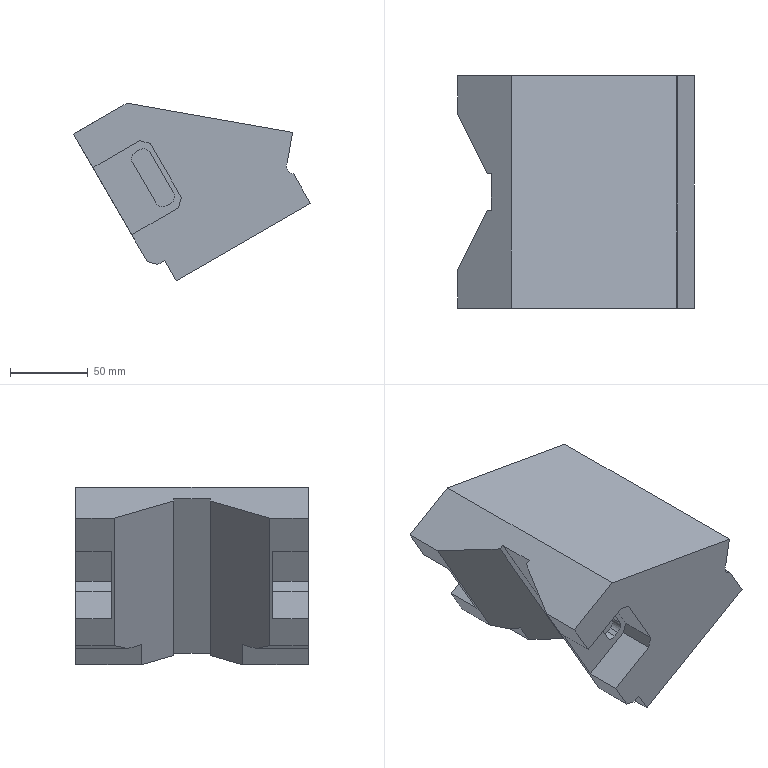Part | NX | features solid 2 | 1 solid | 51 faces | box 152.763 x 150 x 114.501 mm | volume 1337882 mm3 | plane 42 | cylinder 9 | commonest cylinder face diameters 10 x9